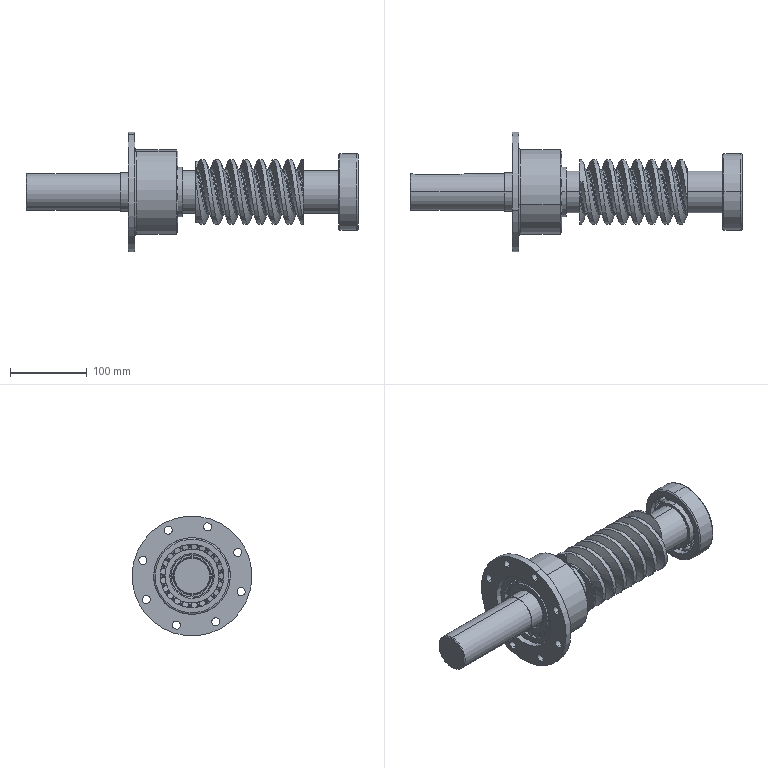Part | SolidWorks | 19 solids | 644 faces | box 432 x 156 x 156 mm | volume 1680982 mm3 | torus 200 | plane 138 | cone 108 | sphere 96 | cylinder 90 | spline 12 | commonest cylinder face diameters 84 x18 10.55 x16 55 x10 100 x8 45 x4 63.4 x4